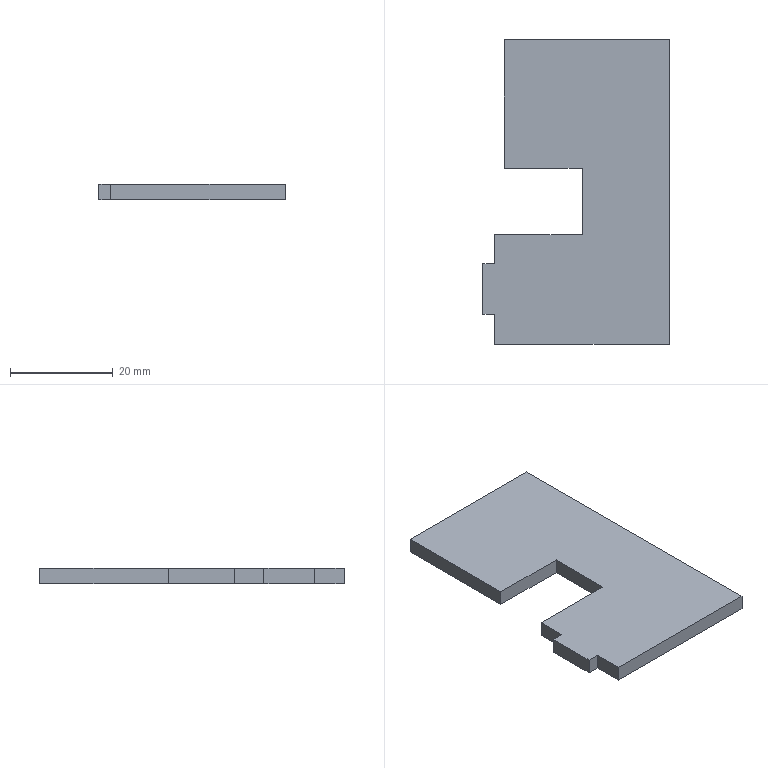Part | SolidWorks | features Extrusion 1 | 1 solid | 14 faces | box 36.242 x 59.193 x 3 mm | volume 5296 mm3 | plane 14
STEP:
#1=CARTESIAN_POINT('',(3.,-12.895,0.));
#2=VERTEX_POINT('',#1);
#3=CARTESIAN_POINT('',(3.,-18.584,0.));
#4=VERTEX_POINT('',#3);
#5=CARTESIAN_POINT('',(3.,-18.584,0.));
#6=DIRECTION('',(0.,-1.,0.));
#7=VECTOR('',#6,1000.);
#8=LINE('',#5,#7);
#9=EDGE_CURVE('',#2,#4,#8,.T.);
#10=ORIENTED_EDGE('',*,*,#9,.T.);
#11=CARTESIAN_POINT('',(3.,-18.584,3.));
#12=VERTEX_POINT('',#11);
#13=CARTESIAN_POINT('',(3.,-18.584,3.));
#14=DIRECTION('',(0.,0.,-1.));
#15=VECTOR('',#14,1000.);
#16=LINE('',#13,#15);
#17=EDGE_CURVE('',#12,#4,#16,.T.);
#18=ORIENTED_EDGE('',*,*,#17,.F.);
#19=CARTESIAN_POINT('',(3.,-12.895,3.));
#20=VERTEX_POINT('',#19);
#21=CARTESIAN_POINT('',(3.,-18.584,3.));
#22=DIRECTION('',(0.,-1.,0.));
#23=VECTOR('',#22,1000.);
#24=LINE('',#21,#23);
#25=EDGE_CURVE('',#20,#12,#24,.T.);
#26=ORIENTED_EDGE('',*,*,#25,.F.);
#27=CARTESIAN_POINT('',(3.,-12.895,3.));
#28=DIRECTION('',(0.,0.,-1.));
#29=VECTOR('',#28,1000.);
#30=LINE('',#27,#29);
#31=EDGE_CURVE('',#20,#2,#30,.T.);
#32=ORIENTED_EDGE('',*,*,#31,.T.);
#33=EDGE_LOOP('',(#10,#18,#26,#32));
#34=FACE_OUTER_BOUND('',#33,.T.);
#35=CARTESIAN_POINT('',(3.,-18.584,3.));
#36=DIRECTION('',(1.,0.,0.));
#37=DIRECTION('',(0.,0.,-1.));
#38=AXIS2_PLACEMENT_3D('',#35,#36,#37);
#39=PLANE('',#38);
#40=ADVANCED_FACE('',(#34),#39,.F.);
#41=CARTESIAN_POINT('',(0.6808,-18.584,0.));
#42=VERTEX_POINT('',#41);
#43=CARTESIAN_POINT('',(3.,-18.584,0.));
#44=DIRECTION('',(-1.,0.,0.));
#45=VECTOR('',#44,1000.);
#46=LINE('',#43,#45);
#47=EDGE_CURVE('',#4,#42,#46,.T.);
#48=ORIENTED_EDGE('',*,*,#47,.T.);
#49=CARTESIAN_POINT('',(0.6808,-18.584,3.));
#50=VERTEX_POINT('',#49);
#51=CARTESIAN_POINT('',(0.6808,-18.584,3.));
#52=DIRECTION('',(0.,0.,-1.));
#53=VECTOR('',#52,1000.);
#54=LINE('',#51,#53);
#55=EDGE_CURVE('',#50,#42,#54,.T.);
#56=ORIENTED_EDGE('',*,*,#55,.F.);
#57=CARTESIAN_POINT('',(3.,-18.584,3.));
#58=DIRECTION('',(-1.,0.,0.));
#59=VECTOR('',#58,1000.);
#60=LINE('',#57,#59);
#61=EDGE_CURVE('',#12,#50,#60,.T.);
#62=ORIENTED_EDGE('',*,*,#61,.F.);
#63=ORIENTED_EDGE('',*,*,#17,.T.);
#64=EDGE_LOOP('',(#48,#56,#62,#63));
#65=FACE_OUTER_BOUND('',#64,.T.);
#66=CARTESIAN_POINT('',(3.,-18.584,3.));
#67=DIRECTION('',(0.,-1.,0.));
#68=DIRECTION('',(0.,0.,-1.));
#69=AXIS2_PLACEMENT_3D('',#66,#67,#68);
#70=PLANE('',#69);
#71=ADVANCED_FACE('',(#65),#70,.F.);
#72=CARTESIAN_POINT('',(0.6808,-28.385,0.));
#73=VERTEX_POINT('',#72);
#74=CARTESIAN_POINT('',(0.6808,-18.584,0.));
#75=DIRECTION('',(0.,-1.,0.));
#76=VECTOR('',#75,1000.);
#77=LINE('',#74,#76);
#78=EDGE_CURVE('',#42,#73,#77,.T.);
#79=ORIENTED_EDGE('',*,*,#78,.T.);
#80=CARTESIAN_POINT('',(0.6808,-28.385,3.));
#81=VERTEX_POINT('',#80);
#82=CARTESIAN_POINT('',(0.6808,-28.385,3.));
#83=DIRECTION('',(0.,0.,-1.));
#84=VECTOR('',#83,1000.);
#85=LINE('',#82,#84);
#86=EDGE_CURVE('',#81,#73,#85,.T.);
#87=ORIENTED_EDGE('',*,*,#86,.F.);
#88=CARTESIAN_POINT('',(0.6808,-18.584,3.));
#89=DIRECTION('',(0.,-1.,0.));
#90=VECTOR('',#89,1000.);
#91=LINE('',#88,#90);
#92=EDGE_CURVE('',#50,#81,#91,.T.);
#93=ORIENTED_EDGE('',*,*,#92,.F.);
#94=ORIENTED_EDGE('',*,*,#55,.T.);
#95=EDGE_LOOP('',(#79,#87,#93,#94));
#96=FACE_OUTER_BOUND('',#95,.T.);
#97=CARTESIAN_POINT('',(0.6808,-18.584,3.));
#98=DIRECTION('',(1.,0.,0.));
#99=DIRECTION('',(0.,0.,-1.));
#100=AXIS2_PLACEMENT_3D('',#97,#98,#99);
#101=PLANE('',#100);
#102=ADVANCED_FACE('',(#96),#101,.F.);
#103=CARTESIAN_POINT('',(3.,-28.385,0.));
#104=VERTEX_POINT('',#103);
#105=CARTESIAN_POINT('',(0.6808,-28.385,0.));
#106=DIRECTION('',(1.,0.,0.));
#107=VECTOR('',#106,1000.);
#108=LINE('',#105,#107);
#109=EDGE_CURVE('',#73,#104,#108,.T.);
#110=ORIENTED_EDGE('',*,*,#109,.T.);
#111=CARTESIAN_POINT('',(3.,-28.385,3.));
#112=VERTEX_POINT('',#111);
#113=CARTESIAN_POINT('',(3.,-28.385,3.));
#114=DIRECTION('',(0.,0.,-1.));
#115=VECTOR('',#114,1000.);
#116=LINE('',#113,#115);
#117=EDGE_CURVE('',#112,#104,#116,.T.);
#118=ORIENTED_EDGE('',*,*,#117,.F.);
#119=CARTESIAN_POINT('',(0.6808,-28.385,3.));
#120=DIRECTION('',(1.,0.,0.));
#121=VECTOR('',#120,1000.);
#122=LINE('',#119,#121);
#123=EDGE_CURVE('',#81,#112,#122,.T.);
#124=ORIENTED_EDGE('',*,*,#123,.F.);
#125=ORIENTED_EDGE('',*,*,#86,.T.);
#126=EDGE_LOOP('',(#110,#118,#124,#125));
#127=FACE_OUTER_BOUND('',#126,.T.);
#128=CARTESIAN_POINT('',(0.6808,-28.385,3.));
#129=DIRECTION('',(0.,1.,0.));
#130=DIRECTION('',(0.,0.,1.));
#131=AXIS2_PLACEMENT_3D('',#128,#129,#130);
#132=PLANE('',#131);
#133=ADVANCED_FACE('',(#127),#132,.F.);
#134=CARTESIAN_POINT('',(3.,-34.193,0.));
#135=VERTEX_POINT('',#134);
#136=CARTESIAN_POINT('',(3.,-28.385,0.));
#137=DIRECTION('',(0.,-1.,0.));
#138=VECTOR('',#137,1000.);
#139=LINE('',#136,#138);
#140=EDGE_CURVE('',#104,#135,#139,.T.);
#141=ORIENTED_EDGE('',*,*,#140,.T.);
#142=CARTESIAN_POINT('',(3.,-34.193,3.));
#143=VERTEX_POINT('',#142);
#144=CARTESIAN_POINT('',(3.,-34.193,3.));
#145=DIRECTION('',(0.,0.,-1.));
#146=VECTOR('',#145,1000.);
#147=LINE('',#144,#146);
#148=EDGE_CURVE('',#143,#135,#147,.T.);
#149=ORIENTED_EDGE('',*,*,#148,.F.);
#150=CARTESIAN_POINT('',(3.,-28.385,3.));
#151=DIRECTION('',(0.,-1.,0.));
#152=VECTOR('',#151,1000.);
#153=LINE('',#150,#152);
#154=EDGE_CURVE('',#112,#143,#153,.T.);
#155=ORIENTED_EDGE('',*,*,#154,.F.);
#156=ORIENTED_EDGE('',*,*,#117,.T.);
#157=EDGE_LOOP('',(#141,#149,#155,#156));
#158=FACE_OUTER_BOUND('',#157,.T.);
#159=CARTESIAN_POINT('',(3.,-28.385,3.));
#160=DIRECTION('',(1.,0.,0.));
#161=DIRECTION('',(0.,0.,-1.));
#162=AXIS2_PLACEMENT_3D('',#159,#160,#161);
#163=PLANE('',#162);
#164=ADVANCED_FACE('',(#158),#163,.F.);
#165=CARTESIAN_POINT('',(36.923,-34.193,0.));
#166=VERTEX_POINT('',#165);
#167=CARTESIAN_POINT('',(3.,-34.193,0.));
#168=DIRECTION('',(1.,0.,0.));
#169=VECTOR('',#168,1000.);
#170=LINE('',#167,#169);
#171=EDGE_CURVE('',#135,#166,#170,.T.);
#172=ORIENTED_EDGE('',*,*,#171,.T.);
#173=CARTESIAN_POINT('',(36.923,-34.193,3.));
#174=VERTEX_POINT('',#173);
#175=CARTESIAN_POINT('',(36.923,-34.193,3.));
#176=DIRECTION('',(0.,0.,-1.));
#177=VECTOR('',#176,1000.);
#178=LINE('',#175,#177);
#179=EDGE_CURVE('',#174,#166,#178,.T.);
#180=ORIENTED_EDGE('',*,*,#179,.F.);
#181=CARTESIAN_POINT('',(3.,-34.193,3.));
#182=DIRECTION('',(1.,0.,0.));
#183=VECTOR('',#182,1000.);
#184=LINE('',#181,#183);
#185=EDGE_CURVE('',#143,#174,#184,.T.);
#186=ORIENTED_EDGE('',*,*,#185,.F.);
#187=ORIENTED_EDGE('',*,*,#148,.T.);
#188=EDGE_LOOP('',(#172,#180,#186,#187));
#189=FACE_OUTER_BOUND('',#188,.T.);
#190=CARTESIAN_POINT('',(3.,-34.193,3.));
#191=DIRECTION('',(0.,1.,0.));
#192=DIRECTION('',(0.,0.,1.));
#193=AXIS2_PLACEMENT_3D('',#190,#191,#192);
#194=PLANE('',#193);
#195=ADVANCED_FACE('',(#189),#194,.F.);
#196=CARTESIAN_POINT('',(36.923,25.,0.));
#197=VERTEX_POINT('',#196);
#198=CARTESIAN_POINT('',(36.923,25.,0.));
#199=DIRECTION('',(0.,1.,0.));
#200=VECTOR('',#199,1000.);
#201=LINE('',#198,#200);
#202=EDGE_CURVE('',#166,#197,#201,.T.);
#203=ORIENTED_EDGE('',*,*,#202,.T.);
#204=CARTESIAN_POINT('',(36.923,25.,3.));
#205=VERTEX_POINT('',#204);
#206=CARTESIAN_POINT('',(36.923,25.,3.));
#207=DIRECTION('',(0.,0.,-1.));
#208=VECTOR('',#207,1000.);
#209=LINE('',#206,#208);
#210=EDGE_CURVE('',#205,#197,#209,.T.);
#211=ORIENTED_EDGE('',*,*,#210,.F.);
#212=CARTESIAN_POINT('',(36.923,25.,3.));
#213=DIRECTION('',(0.,1.,0.));
#214=VECTOR('',#213,1000.);
#215=LINE('',#212,#214);
#216=EDGE_CURVE('',#174,#205,#215,.T.);
#217=ORIENTED_EDGE('',*,*,#216,.F.);
#218=ORIENTED_EDGE('',*,*,#179,.T.);
#219=EDGE_LOOP('',(#203,#211,#217,#218));
#220=FACE_OUTER_BOUND('',#219,.T.);
#221=CARTESIAN_POINT('',(36.923,25.,3.));
#222=DIRECTION('',(-1.,0.,0.));
#223=DIRECTION('',(0.,0.,1.));
#224=AXIS2_PLACEMENT_3D('',#221,#222,#223);
#225=PLANE('',#224);
#226=ADVANCED_FACE('',(#220),#225,.F.);
#227=CARTESIAN_POINT('',(4.847,25.,0.));
#228=VERTEX_POINT('',#227);
#229=CARTESIAN_POINT('',(4.847,25.,0.));
#230=DIRECTION('',(-1.,0.,0.));
#231=VECTOR('',#230,1000.);
#232=LINE('',#229,#231);
#233=EDGE_CURVE('',#197,#228,#232,.T.);
#234=ORIENTED_EDGE('',*,*,#233,.T.);
#235=CARTESIAN_POINT('',(4.847,25.,3.));
#236=VERTEX_POINT('',#235);
#237=CARTESIAN_POINT('',(4.847,25.,3.));
#238=DIRECTION('',(0.,0.,-1.));
#239=VECTOR('',#238,1000.);
#240=LINE('',#237,#239);
#241=EDGE_CURVE('',#236,#228,#240,.T.);
#242=ORIENTED_EDGE('',*,*,#241,.F.);
#243=CARTESIAN_POINT('',(4.847,25.,3.));
#244=DIRECTION('',(-1.,0.,0.));
#245=VECTOR('',#244,1000.);
#246=LINE('',#243,#245);
#247=EDGE_CURVE('',#205,#236,#246,.T.);
#248=ORIENTED_EDGE('',*,*,#247,.F.);
#249=ORIENTED_EDGE('',*,*,#210,.T.);
#250=EDGE_LOOP('',(#234,#242,#248,#249));
#251=FACE_OUTER_BOUND('',#250,.T.);
#252=CARTESIAN_POINT('',(4.847,25.,3.));
#253=DIRECTION('',(0.,-1.,0.));
#254=DIRECTION('',(0.,0.,-1.));
#255=AXIS2_PLACEMENT_3D('',#252,#253,#254);
#256=PLANE('',#255);
#257=ADVANCED_FACE('',(#251),#256,.F.);
#258=CARTESIAN_POINT('',(4.847,0.,0.));
#259=VERTEX_POINT('',#258);
#260=CARTESIAN_POINT('',(4.847,0.,0.));
#261=DIRECTION('',(0.,-1.,0.));
#262=VECTOR('',#261,1000.);
#263=LINE('',#260,#262);
#264=EDGE_CURVE('',#228,#259,#263,.T.);
#265=ORIENTED_EDGE('',*,*,#264,.T.);
#266=CARTESIAN_POINT('',(4.847,0.,3.));
#267=VERTEX_POINT('',#266);
#268=CARTESIAN_POINT('',(4.847,0.,3.));
#269=DIRECTION('',(0.,0.,-1.));
#270=VECTOR('',#269,1000.);
#271=LINE('',#268,#270);
#272=EDGE_CURVE('',#267,#259,#271,.T.);
#273=ORIENTED_EDGE('',*,*,#272,.F.);
#274=CARTESIAN_POINT('',(4.847,0.,3.));
#275=DIRECTION('',(0.,-1.,0.));
#276=VECTOR('',#275,1000.);
#277=LINE('',#274,#276);
#278=EDGE_CURVE('',#236,#267,#277,.T.);
#279=ORIENTED_EDGE('',*,*,#278,.F.);
#280=ORIENTED_EDGE('',*,*,#241,.T.);
#281=EDGE_LOOP('',(#265,#273,#279,#280));
#282=FACE_OUTER_BOUND('',#281,.T.);
#283=CARTESIAN_POINT('',(4.847,0.,3.));
#284=DIRECTION('',(1.,0.,0.));
#285=DIRECTION('',(0.,0.,-1.));
#286=AXIS2_PLACEMENT_3D('',#283,#284,#285);
#287=PLANE('',#286);
#288=ADVANCED_FACE('',(#282),#287,.F.);
#289=CARTESIAN_POINT('',(20.,0.,0.));
#290=VERTEX_POINT('',#289);
#291=CARTESIAN_POINT('',(20.,0.,0.));
#292=DIRECTION('',(1.,0.,0.));
#293=VECTOR('',#292,1000.);
#294=LINE('',#291,#293);
#295=EDGE_CURVE('',#259,#290,#294,.T.);
#296=ORIENTED_EDGE('',*,*,#295,.T.);
#297=CARTESIAN_POINT('',(20.,0.,3.));
#298=VERTEX_POINT('',#297);
#299=CARTESIAN_POINT('',(20.,0.,3.));
#300=DIRECTION('',(0.,0.,-1.));
#301=VECTOR('',#300,1000.);
#302=LINE('',#299,#301);
#303=EDGE_CURVE('',#298,#290,#302,.T.);
#304=ORIENTED_EDGE('',*,*,#303,.F.);
#305=CARTESIAN_POINT('',(20.,0.,3.));
#306=DIRECTION('',(1.,0.,0.));
#307=VECTOR('',#306,1000.);
#308=LINE('',#305,#307);
#309=EDGE_CURVE('',#267,#298,#308,.T.);
#310=ORIENTED_EDGE('',*,*,#309,.F.);
#311=ORIENTED_EDGE('',*,*,#272,.T.);
#312=EDGE_LOOP('',(#296,#304,#310,#311));
#313=FACE_OUTER_BOUND('',#312,.T.);
#314=CARTESIAN_POINT('',(20.,0.,3.));
#315=DIRECTION('',(0.,1.,0.));
#316=DIRECTION('',(0.,0.,1.));
#317=AXIS2_PLACEMENT_3D('',#314,#315,#316);
#318=PLANE('',#317);
#319=ADVANCED_FACE('',(#313),#318,.F.);
#320=CARTESIAN_POINT('',(20.,-12.895,0.));
#321=VERTEX_POINT('',#320);
#322=CARTESIAN_POINT('',(20.,-12.895,0.));
#323=DIRECTION('',(0.,-1.,0.));
#324=VECTOR('',#323,1000.);
#325=LINE('',#322,#324);
#326=EDGE_CURVE('',#290,#321,#325,.T.);
#327=ORIENTED_EDGE('',*,*,#326,.T.);
#328=CARTESIAN_POINT('',(20.,-12.895,3.));
#329=VERTEX_POINT('',#328);
#330=CARTESIAN_POINT('',(20.,-12.895,3.));
#331=DIRECTION('',(0.,0.,-1.));
#332=VECTOR('',#331,1000.);
#333=LINE('',#330,#332);
#334=EDGE_CURVE('',#329,#321,#333,.T.);
#335=ORIENTED_EDGE('',*,*,#334,.F.);
#336=CARTESIAN_POINT('',(20.,-12.895,3.));
#337=DIRECTION('',(0.,-1.,0.));
#338=VECTOR('',#337,1000.);
#339=LINE('',#336,#338);
#340=EDGE_CURVE('',#298,#329,#339,.T.);
#341=ORIENTED_EDGE('',*,*,#340,.F.);
#342=ORIENTED_EDGE('',*,*,#303,.T.);
#343=EDGE_LOOP('',(#327,#335,#341,#342));
#344=FACE_OUTER_BOUND('',#343,.T.);
#345=CARTESIAN_POINT('',(20.,-12.895,3.));
#346=DIRECTION('',(1.,0.,0.));
#347=DIRECTION('',(0.,0.,-1.));
#348=AXIS2_PLACEMENT_3D('',#345,#346,#347);
#349=PLANE('',#348);
#350=ADVANCED_FACE('',(#344),#349,.F.);
#351=CARTESIAN_POINT('',(3.,-12.895,0.));
#352=DIRECTION('',(-1.,0.,0.));
#353=VECTOR('',#352,1000.);
#354=LINE('',#351,#353);
#355=EDGE_CURVE('',#321,#2,#354,.T.);
#356=ORIENTED_EDGE('',*,*,#355,.T.);
#357=ORIENTED_EDGE('',*,*,#31,.F.);
#358=CARTESIAN_POINT('',(3.,-12.895,3.));
#359=DIRECTION('',(-1.,0.,0.));
#360=VECTOR('',#359,1000.);
#361=LINE('',#358,#360);
#362=EDGE_CURVE('',#329,#20,#361,.T.);
#363=ORIENTED_EDGE('',*,*,#362,.F.);
#364=ORIENTED_EDGE('',*,*,#334,.T.);
#365=EDGE_LOOP('',(#356,#357,#363,#364));
#366=FACE_OUTER_BOUND('',#365,.T.);
#367=CARTESIAN_POINT('',(3.,-12.895,3.));
#368=DIRECTION('',(0.,-1.,0.));
#369=DIRECTION('',(1.,0.,0.));
#370=AXIS2_PLACEMENT_3D('',#367,#368,#369);
#371=PLANE('',#370);
#372=ADVANCED_FACE('',(#366),#371,.F.);
#373=ORIENTED_EDGE('',*,*,#25,.T.);
#374=ORIENTED_EDGE('',*,*,#61,.T.);
#375=ORIENTED_EDGE('',*,*,#92,.T.);
#376=ORIENTED_EDGE('',*,*,#123,.T.);
#377=ORIENTED_EDGE('',*,*,#154,.T.);
#378=ORIENTED_EDGE('',*,*,#185,.T.);
#379=ORIENTED_EDGE('',*,*,#216,.T.);
#380=ORIENTED_EDGE('',*,*,#247,.T.);
#381=ORIENTED_EDGE('',*,*,#278,.T.);
#382=ORIENTED_EDGE('',*,*,#309,.T.);
#383=ORIENTED_EDGE('',*,*,#340,.T.);
#384=ORIENTED_EDGE('',*,*,#362,.T.);
#385=EDGE_LOOP('',(#373,#374,#375,#376,#377,#378,#379,#380,#381,#382,#383,#384));
#386=FACE_OUTER_BOUND('',#385,.T.);
#387=CARTESIAN_POINT('',(0.,0.,3.));
#388=DIRECTION('',(0.,0.,-1.));
#389=DIRECTION('',(-1.,0.,0.));
#390=AXIS2_PLACEMENT_3D('',#387,#388,#389);
#391=PLANE('',#390);
#392=ADVANCED_FACE('',(#386),#391,.F.);
#393=ORIENTED_EDGE('',*,*,#9,.F.);
#394=ORIENTED_EDGE('',*,*,#355,.F.);
#395=ORIENTED_EDGE('',*,*,#326,.F.);
#396=ORIENTED_EDGE('',*,*,#295,.F.);
#397=ORIENTED_EDGE('',*,*,#264,.F.);
#398=ORIENTED_EDGE('',*,*,#233,.F.);
#399=ORIENTED_EDGE('',*,*,#202,.F.);
#400=ORIENTED_EDGE('',*,*,#171,.F.);
#401=ORIENTED_EDGE('',*,*,#140,.F.);
#402=ORIENTED_EDGE('',*,*,#109,.F.);
#403=ORIENTED_EDGE('',*,*,#78,.F.);
#404=ORIENTED_EDGE('',*,*,#47,.F.);
#405=EDGE_LOOP('',(#393,#394,#395,#396,#397,#398,#399,#400,#401,#402,#403,#404));
#406=FACE_OUTER_BOUND('',#405,.T.);
#407=CARTESIAN_POINT('',(0.,0.,0.));
#408=DIRECTION('',(0.,0.,-1.));
#409=DIRECTION('',(-1.,0.,0.));
#410=AXIS2_PLACEMENT_3D('',#407,#408,#409);
#411=PLANE('',#410);
#412=ADVANCED_FACE('',(#406),#411,.T.);
#413=CLOSED_SHELL('',(#40,#71,#102,#133,#164,#195,#226,#257,#288,#319,#350,#372,#392,#412));
#414=MANIFOLD_SOLID_BREP('',#413);
#415=CARTESIAN_POINT('',(0.,0.,0.));
#416=DIRECTION('',(0.,0.,1.));
#417=DIRECTION('',(1.,0.,0.));
#418=AXIS2_PLACEMENT_3D('',#415,#416,#417);
#419=(LENGTH_UNIT()NAMED_UNIT(*)SI_UNIT(.MILLI.,.METRE.));
#420=UNCERTAINTY_MEASURE_WITH_UNIT(LENGTH_MEASURE(0.00001),#419,'','');
#421=(NAMED_UNIT(*)PLANE_ANGLE_UNIT()SI_UNIT($,.RADIAN.));
#422=(NAMED_UNIT(*)SI_UNIT($,.STERADIAN.)SOLID_ANGLE_UNIT());
#423=(GEOMETRIC_REPRESENTATION_CONTEXT(3)GLOBAL_UNCERTAINTY_ASSIGNED_CONTEXT((#420))GLOBAL_UNIT_ASSIGNED_CONTEXT((#419,#421,#422))REPRESENTATION_CONTEXT('',''));
#424=ADVANCED_BREP_SHAPE_REPRESENTATION('',(#414,#418),#423);